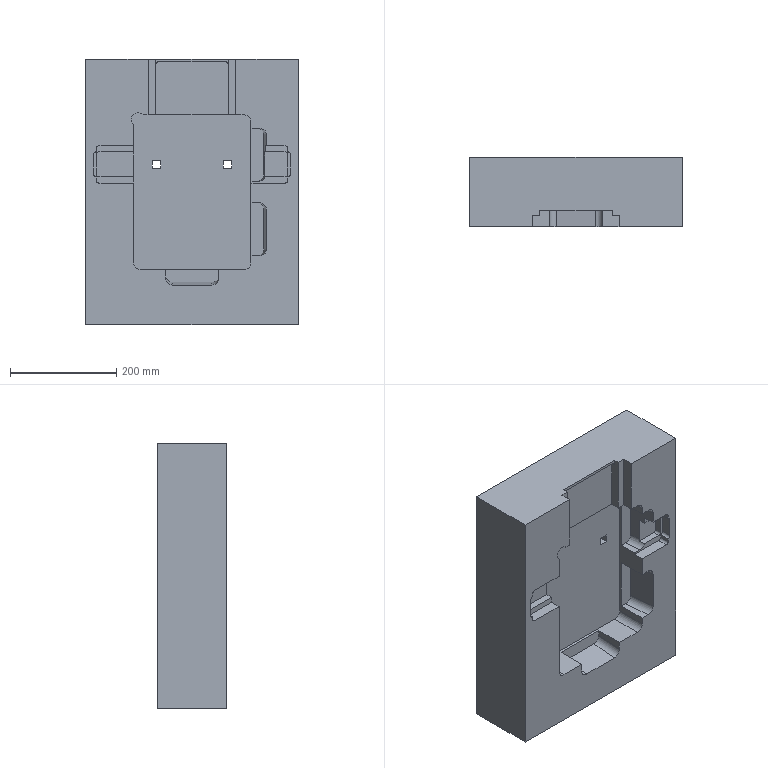Part | STEP file | 1 solid | 92 faces | box 400 x 130 x 500 mm | volume 20837897 mm3 | plane 64 | cylinder 28 | commonest cylinder face diameters 10 x18 26 x10